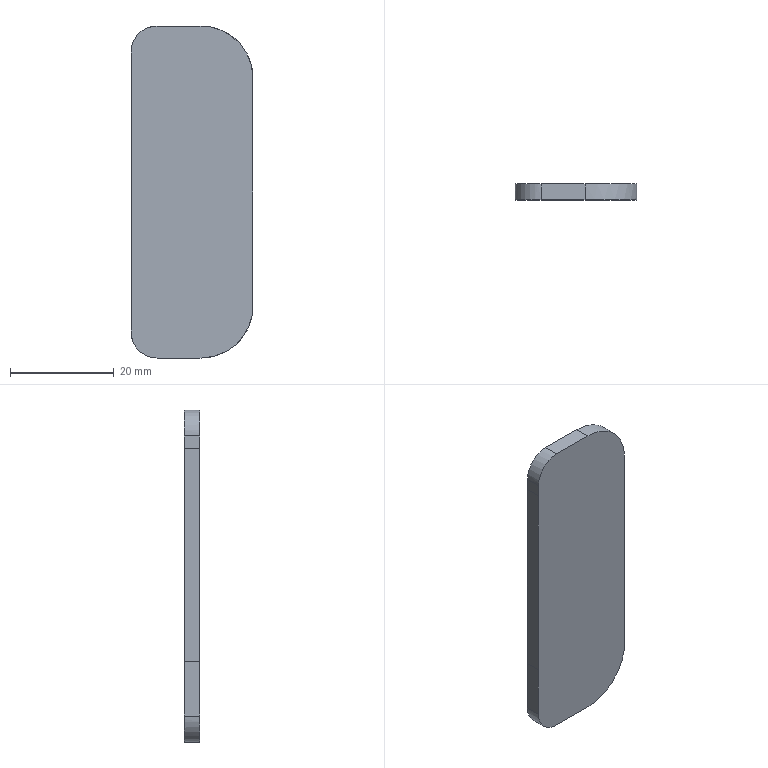Part | NX | features BREP 1 | 1 solid | 12 faces | volume 4337 mm3 | plane 8 | cylinder 4 | commonest cylinder face diameters 10 x2 20 x2